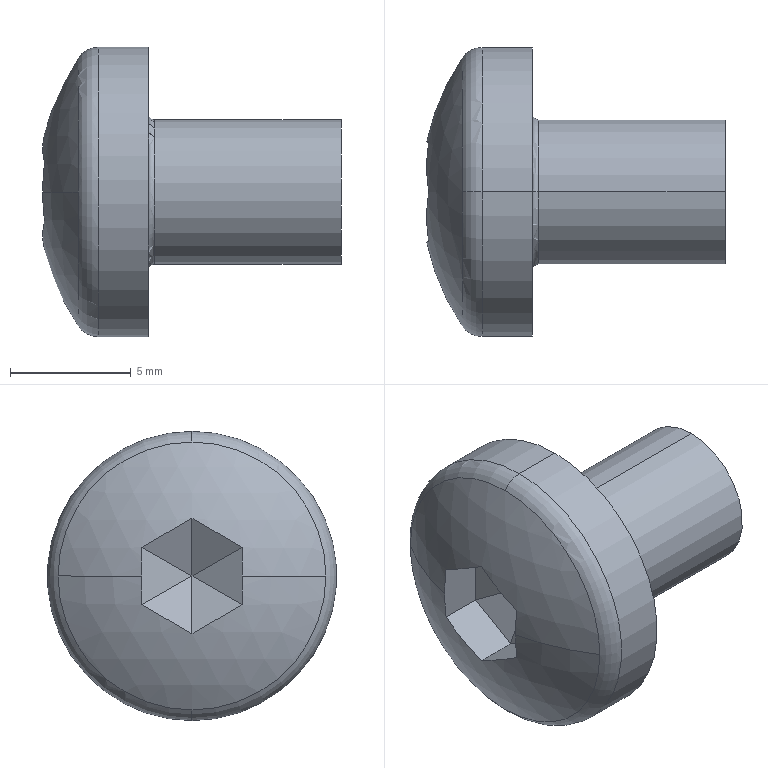Part | SolidWorks | features Cut 2, Fillet 2, RevCut 2, Boss 1, Extrusion 1, LPattern 1 | 1 solid | 24 faces | box 12.382 x 12 x 12 mm | volume 602.281 mm3 | plane 14 | torus 4 | cylinder 4 | sphere 2 | commonest cylinder face diameters 6 x2 12 x2
STEP:
#1=CARTESIAN_POINT('',(1.685,0.,5.556));
#2=VERTEX_POINT('',#1);
#3=CARTESIAN_POINT('',(1.685,5.556,0.));
#4=VERTEX_POINT('',#3);
#5=CARTESIAN_POINT('',(1.685,0.,0.));
#6=DIRECTION('',(-1.,0.,0.));
#7=DIRECTION('',(0.,0.,-1.));
#8=AXIS2_PLACEMENT_3D('',#5,#6,#7);
#9=CIRCLE('',#8,5.556);
#10=EDGE_CURVE('',#2,#4,#9,.T.);
#11=ORIENTED_EDGE('',*,*,#10,.F.);
#12=CARTESIAN_POINT('',(2.517,0.,6.));
#13=VERTEX_POINT('',#12);
#14=CARTESIAN_POINT('',(2.517,0.,5.));
#15=DIRECTION('',(0.,1.,0.));
#16=DIRECTION('',(0.,0.,1.));
#17=AXIS2_PLACEMENT_3D('',#14,#15,#16);
#18=CIRCLE('',#17,1.);
#19=EDGE_CURVE('',#2,#13,#18,.T.);
#20=ORIENTED_EDGE('',*,*,#19,.T.);
#21=CARTESIAN_POINT('',(2.517,0.,-6.));
#22=VERTEX_POINT('',#21);
#23=CARTESIAN_POINT('',(2.517,0.,0.));
#24=DIRECTION('',(1.,0.,0.));
#25=DIRECTION('',(0.,0.,-1.));
#26=AXIS2_PLACEMENT_3D('',#23,#24,#25);
#27=CIRCLE('',#26,6.);
#28=EDGE_CURVE('',#22,#13,#27,.T.);
#29=ORIENTED_EDGE('',*,*,#28,.F.);
#30=CARTESIAN_POINT('',(1.685,0.,-5.556));
#31=VERTEX_POINT('',#30);
#32=CARTESIAN_POINT('',(2.517,0.,-5.));
#33=DIRECTION('',(0.,-1.,0.));
#34=DIRECTION('',(0.,0.,-1.));
#35=AXIS2_PLACEMENT_3D('',#32,#33,#34);
#36=CIRCLE('',#35,1.);
#37=EDGE_CURVE('',#31,#22,#36,.T.);
#38=ORIENTED_EDGE('',*,*,#37,.F.);
#39=CARTESIAN_POINT('',(1.685,0.,0.));
#40=DIRECTION('',(-1.,0.,0.));
#41=DIRECTION('',(0.,0.,-1.));
#42=AXIS2_PLACEMENT_3D('',#39,#40,#41);
#43=CIRCLE('',#42,5.556);
#44=EDGE_CURVE('',#4,#31,#43,.T.);
#45=ORIENTED_EDGE('',*,*,#44,.F.);
#46=EDGE_LOOP('',(#11,#20,#29,#38,#45));
#47=FACE_OUTER_BOUND('',#46,.T.);
#48=CARTESIAN_POINT('',(2.517,0.,0.));
#49=DIRECTION('',(1.,0.,0.));
#50=DIRECTION('',(0.,0.,-1.));
#51=AXIS2_PLACEMENT_3D('',#48,#49,#50);
#52=TOROIDAL_SURFACE('',#51,5.,1.);
#53=ADVANCED_FACE('',(#47),#52,.T.);
#54=CARTESIAN_POINT('',(4.85,0.,3.));
#55=VERTEX_POINT('',#54);
#56=CARTESIAN_POINT('',(4.85,0.,-3.));
#57=VERTEX_POINT('',#56);
#58=CARTESIAN_POINT('',(4.85,0.,0.));
#59=DIRECTION('',(1.,0.,0.));
#60=DIRECTION('',(0.,0.,-1.));
#61=AXIS2_PLACEMENT_3D('',#58,#59,#60);
#62=CIRCLE('',#61,3.);
#63=EDGE_CURVE('',#55,#57,#62,.T.);
#64=ORIENTED_EDGE('',*,*,#63,.F.);
#65=CARTESIAN_POINT('',(4.6,0.,3.25));
#66=VERTEX_POINT('',#65);
#67=CARTESIAN_POINT('',(4.85,0.,3.25));
#68=DIRECTION('',(0.,1.,0.));
#69=DIRECTION('',(0.,0.,1.));
#70=AXIS2_PLACEMENT_3D('',#67,#68,#69);
#71=CIRCLE('',#70,0.25);
#72=EDGE_CURVE('',#55,#66,#71,.T.);
#73=ORIENTED_EDGE('',*,*,#72,.T.);
#74=CARTESIAN_POINT('',(4.6,0.,-3.25));
#75=VERTEX_POINT('',#74);
#76=CARTESIAN_POINT('',(4.6,0.,0.));
#77=DIRECTION('',(-1.,0.,0.));
#78=DIRECTION('',(0.,0.,-1.));
#79=AXIS2_PLACEMENT_3D('',#76,#77,#78);
#80=CIRCLE('',#79,3.25);
#81=EDGE_CURVE('',#75,#66,#80,.T.);
#82=ORIENTED_EDGE('',*,*,#81,.F.);
#83=CARTESIAN_POINT('',(4.85,0.,-3.25));
#84=DIRECTION('',(0.,-1.,0.));
#85=DIRECTION('',(0.,0.,-1.));
#86=AXIS2_PLACEMENT_3D('',#83,#84,#85);
#87=CIRCLE('',#86,0.25);
#88=EDGE_CURVE('',#57,#75,#87,.T.);
#89=ORIENTED_EDGE('',*,*,#88,.F.);
#90=EDGE_LOOP('',(#64,#73,#82,#89));
#91=FACE_OUTER_BOUND('',#90,.T.);
#92=CARTESIAN_POINT('',(4.85,0.,0.));
#93=DIRECTION('',(1.,0.,0.));
#94=DIRECTION('',(0.,0.,-1.));
#95=AXIS2_PLACEMENT_3D('',#92,#93,#94);
#96=TOROIDAL_SURFACE('',#95,3.25,0.25);
#97=ADVANCED_FACE('',(#91),#96,.F.);
#98=CARTESIAN_POINT('',(12.6,0.,-3.));
#99=VERTEX_POINT('',#98);
#100=CARTESIAN_POINT('',(12.6,0.,3.));
#101=VERTEX_POINT('',#100);
#102=CARTESIAN_POINT('',(12.6,0.,0.));
#103=DIRECTION('',(1.,0.,0.));
#104=DIRECTION('',(0.,0.,-1.));
#105=AXIS2_PLACEMENT_3D('',#102,#103,#104);
#106=CIRCLE('',#105,3.);
#107=EDGE_CURVE('',#99,#101,#106,.T.);
#108=ORIENTED_EDGE('',*,*,#107,.F.);
#109=CARTESIAN_POINT('',(12.6,0.,-3.));
#110=DIRECTION('',(-1.,0.,0.));
#111=VECTOR('',#110,1000.);
#112=LINE('',#109,#111);
#113=EDGE_CURVE('',#99,#57,#112,.T.);
#114=ORIENTED_EDGE('',*,*,#113,.T.);
#115=CARTESIAN_POINT('',(4.85,0.,0.));
#116=DIRECTION('',(1.,0.,0.));
#117=DIRECTION('',(0.,0.,-1.));
#118=AXIS2_PLACEMENT_3D('',#115,#116,#117);
#119=CIRCLE('',#118,3.);
#120=EDGE_CURVE('',#57,#55,#119,.T.);
#121=ORIENTED_EDGE('',*,*,#120,.T.);
#122=CARTESIAN_POINT('',(12.6,0.,3.));
#123=DIRECTION('',(-1.,0.,0.));
#124=VECTOR('',#123,1000.);
#125=LINE('',#122,#124);
#126=EDGE_CURVE('',#101,#55,#125,.T.);
#127=ORIENTED_EDGE('',*,*,#126,.F.);
#128=EDGE_LOOP('',(#108,#114,#121,#127));
#129=FACE_OUTER_BOUND('',#128,.T.);
#130=CARTESIAN_POINT('',(12.6,0.,0.));
#131=DIRECTION('',(-1.,0.,0.));
#132=DIRECTION('',(0.,0.,1.));
#133=AXIS2_PLACEMENT_3D('',#130,#131,#132);
#134=CYLINDRICAL_SURFACE('',#133,3.);
#135=ADVANCED_FACE('',(#129),#134,.T.);
#136=CARTESIAN_POINT('',(4.6,0.,-6.));
#137=VERTEX_POINT('',#136);
#138=CARTESIAN_POINT('',(4.6,0.,6.));
#139=VERTEX_POINT('',#138);
#140=CARTESIAN_POINT('',(4.6,0.,0.));
#141=DIRECTION('',(1.,0.,0.));
#142=DIRECTION('',(0.,0.,-1.));
#143=AXIS2_PLACEMENT_3D('',#140,#141,#142);
#144=CIRCLE('',#143,6.);
#145=EDGE_CURVE('',#137,#139,#144,.T.);
#146=ORIENTED_EDGE('',*,*,#145,.F.);
#147=CARTESIAN_POINT('',(4.6,0.,-6.));
#148=DIRECTION('',(-1.,0.,0.));
#149=VECTOR('',#148,1000.);
#150=LINE('',#147,#149);
#151=EDGE_CURVE('',#137,#22,#150,.T.);
#152=ORIENTED_EDGE('',*,*,#151,.T.);
#153=ORIENTED_EDGE('',*,*,#28,.T.);
#154=CARTESIAN_POINT('',(4.6,0.,6.));
#155=DIRECTION('',(-1.,0.,0.));
#156=VECTOR('',#155,1000.);
#157=LINE('',#154,#156);
#158=EDGE_CURVE('',#139,#13,#157,.T.);
#159=ORIENTED_EDGE('',*,*,#158,.F.);
#160=EDGE_LOOP('',(#146,#152,#153,#159));
#161=FACE_OUTER_BOUND('',#160,.T.);
#162=CARTESIAN_POINT('',(4.6,0.,0.));
#163=DIRECTION('',(-1.,0.,0.));
#164=DIRECTION('',(0.,0.,1.));
#165=AXIS2_PLACEMENT_3D('',#162,#163,#164);
#166=CYLINDRICAL_SURFACE('',#165,6.);
#167=ADVANCED_FACE('',(#161),#166,.T.);
#168=CARTESIAN_POINT('',(1.685,-5.556,0.));
#169=VERTEX_POINT('',#168);
#170=CARTESIAN_POINT('',(1.685,0.,0.));
#171=DIRECTION('',(-1.,0.,0.));
#172=DIRECTION('',(0.,0.,-1.));
#173=AXIS2_PLACEMENT_3D('',#170,#171,#172);
#174=CIRCLE('',#173,5.556);
#175=EDGE_CURVE('',#169,#2,#174,.T.);
#176=ORIENTED_EDGE('',*,*,#175,.T.);
#177=ORIENTED_EDGE('',*,*,#10,.T.);
#178=CARTESIAN_POINT('',(0.2176,2.075,0.));
#179=VERTEX_POINT('',#178);
#180=CARTESIAN_POINT('',(10.,0.,0.));
#181=DIRECTION('',(0.,0.,1.));
#182=DIRECTION('',(0.,-1.,0.));
#183=AXIS2_PLACEMENT_3D('',#180,#181,#182);
#184=CIRCLE('',#183,10.);
#185=EDGE_CURVE('',#4,#179,#184,.T.);
#186=ORIENTED_EDGE('',*,*,#185,.T.);
#187=CARTESIAN_POINT('',(0.2913,2.075,1.198));
#188=VERTEX_POINT('',#187);
#189=CARTESIAN_POINT('',(10.,2.075,0.));
#190=DIRECTION('',(0.,1.,0.));
#191=DIRECTION('',(0.,0.,-1.));
#192=AXIS2_PLACEMENT_3D('',#189,#190,#191);
#193=CIRCLE('',#192,9.782);
#194=EDGE_CURVE('',#179,#188,#193,.T.);
#195=ORIENTED_EDGE('',*,*,#194,.T.);
#196=CARTESIAN_POINT('',(0.2913,0.,2.396));
#197=VERTEX_POINT('',#196);
#198=CARTESIAN_POINT('',(10.,1.038,1.797));
#199=DIRECTION('',(0.,0.5,0.866));
#200=DIRECTION('',(0.,0.866,-0.5));
#201=AXIS2_PLACEMENT_3D('',#198,#199,#200);
#202=CIRCLE('',#201,9.782);
#203=EDGE_CURVE('',#188,#197,#202,.T.);
#204=ORIENTED_EDGE('',*,*,#203,.T.);
#205=CARTESIAN_POINT('',(0.2913,-2.075,1.198));
#206=VERTEX_POINT('',#205);
#207=CARTESIAN_POINT('',(10.,-1.037,1.797));
#208=DIRECTION('',(0.,-0.5,0.866));
#209=DIRECTION('',(0.,0.866,0.5));
#210=AXIS2_PLACEMENT_3D('',#207,#208,#209);
#211=CIRCLE('',#210,9.782);
#212=EDGE_CURVE('',#197,#206,#211,.T.);
#213=ORIENTED_EDGE('',*,*,#212,.T.);
#214=CARTESIAN_POINT('',(0.2176,-2.075,0.));
#215=VERTEX_POINT('',#214);
#216=CARTESIAN_POINT('',(10.,-2.075,0.));
#217=DIRECTION('',(0.,-1.,0.));
#218=DIRECTION('',(0.,0.,1.));
#219=AXIS2_PLACEMENT_3D('',#216,#217,#218);
#220=CIRCLE('',#219,9.782);
#221=EDGE_CURVE('',#206,#215,#220,.T.);
#222=ORIENTED_EDGE('',*,*,#221,.T.);
#223=CARTESIAN_POINT('',(10.,0.,0.));
#224=DIRECTION('',(0.,0.,-1.));
#225=DIRECTION('',(-1.,0.,0.));
#226=AXIS2_PLACEMENT_3D('',#223,#224,#225);
#227=CIRCLE('',#226,10.);
#228=EDGE_CURVE('',#169,#215,#227,.T.);
#229=ORIENTED_EDGE('',*,*,#228,.F.);
#230=EDGE_LOOP('',(#176,#177,#186,#195,#204,#213,#222,#229));
#231=FACE_OUTER_BOUND('',#230,.T.);
#232=CARTESIAN_POINT('',(10.,0.,0.));
#233=DIRECTION('',(0.,0.,1.));
#234=DIRECTION('',(0.,-1.,0.));
#235=AXIS2_PLACEMENT_3D('',#232,#233,#234);
#236=SPHERICAL_SURFACE('',#235,10.);
#237=ADVANCED_FACE('',(#231),#236,.T.);
#238=ORIENTED_EDGE('',*,*,#185,.F.);
#239=ORIENTED_EDGE('',*,*,#44,.T.);
#240=CARTESIAN_POINT('',(1.685,0.,0.));
#241=DIRECTION('',(-1.,0.,0.));
#242=DIRECTION('',(0.,0.,-1.));
#243=AXIS2_PLACEMENT_3D('',#240,#241,#242);
#244=CIRCLE('',#243,5.556);
#245=EDGE_CURVE('',#31,#169,#244,.T.);
#246=ORIENTED_EDGE('',*,*,#245,.T.);
#247=ORIENTED_EDGE('',*,*,#228,.T.);
#248=CARTESIAN_POINT('',(0.2913,-2.075,-1.198));
#249=VERTEX_POINT('',#248);
#250=CARTESIAN_POINT('',(10.,-2.075,0.));
#251=DIRECTION('',(0.,-1.,0.));
#252=DIRECTION('',(0.,0.,1.));
#253=AXIS2_PLACEMENT_3D('',#250,#251,#252);
#254=CIRCLE('',#253,9.782);
#255=EDGE_CURVE('',#215,#249,#254,.T.);
#256=ORIENTED_EDGE('',*,*,#255,.T.);
#257=CARTESIAN_POINT('',(0.2913,0.,-2.396));
#258=VERTEX_POINT('',#257);
#259=CARTESIAN_POINT('',(10.,-1.038,-1.797));
#260=DIRECTION('',(0.,-0.5,-0.866));
#261=DIRECTION('',(0.,-0.866,0.5));
#262=AXIS2_PLACEMENT_3D('',#259,#260,#261);
#263=CIRCLE('',#262,9.782);
#264=EDGE_CURVE('',#249,#258,#263,.T.);
#265=ORIENTED_EDGE('',*,*,#264,.T.);
#266=CARTESIAN_POINT('',(0.2913,2.075,-1.198));
#267=VERTEX_POINT('',#266);
#268=CARTESIAN_POINT('',(10.,1.037,-1.797));
#269=DIRECTION('',(0.,0.5,-0.866));
#270=DIRECTION('',(0.,-0.866,-0.5));
#271=AXIS2_PLACEMENT_3D('',#268,#269,#270);
#272=CIRCLE('',#271,9.782);
#273=EDGE_CURVE('',#258,#267,#272,.T.);
#274=ORIENTED_EDGE('',*,*,#273,.T.);
#275=CARTESIAN_POINT('',(10.,2.075,0.));
#276=DIRECTION('',(0.,1.,0.));
#277=DIRECTION('',(0.,0.,-1.));
#278=AXIS2_PLACEMENT_3D('',#275,#276,#277);
#279=CIRCLE('',#278,9.782);
#280=EDGE_CURVE('',#267,#179,#279,.T.);
#281=ORIENTED_EDGE('',*,*,#280,.T.);
#282=EDGE_LOOP('',(#238,#239,#246,#247,#256,#265,#274,#281));
#283=FACE_OUTER_BOUND('',#282,.T.);
#284=CARTESIAN_POINT('',(10.,0.,0.));
#285=DIRECTION('',(0.,0.,1.));
#286=DIRECTION('',(0.,-1.,0.));
#287=AXIS2_PLACEMENT_3D('',#284,#285,#286);
#288=SPHERICAL_SURFACE('',#287,10.);
#289=ADVANCED_FACE('',(#283),#288,.T.);
#290=ORIENTED_EDGE('',*,*,#151,.F.);
#291=CARTESIAN_POINT('',(4.6,0.,0.));
#292=DIRECTION('',(1.,0.,0.));
#293=DIRECTION('',(0.,0.,-1.));
#294=AXIS2_PLACEMENT_3D('',#291,#292,#293);
#295=CIRCLE('',#294,6.);
#296=EDGE_CURVE('',#139,#137,#295,.T.);
#297=ORIENTED_EDGE('',*,*,#296,.F.);
#298=ORIENTED_EDGE('',*,*,#158,.T.);
#299=CARTESIAN_POINT('',(2.517,0.,0.));
#300=DIRECTION('',(1.,0.,0.));
#301=DIRECTION('',(0.,0.,-1.));
#302=AXIS2_PLACEMENT_3D('',#299,#300,#301);
#303=CIRCLE('',#302,6.);
#304=EDGE_CURVE('',#13,#22,#303,.T.);
#305=ORIENTED_EDGE('',*,*,#304,.T.);
#306=EDGE_LOOP('',(#290,#297,#298,#305));
#307=FACE_OUTER_BOUND('',#306,.T.);
#308=CARTESIAN_POINT('',(4.6,0.,0.));
#309=DIRECTION('',(-1.,0.,0.));
#310=DIRECTION('',(0.,0.,1.));
#311=AXIS2_PLACEMENT_3D('',#308,#309,#310);
#312=CYLINDRICAL_SURFACE('',#311,6.);
#313=ADVANCED_FACE('',(#307),#312,.T.);
#314=ORIENTED_EDGE('',*,*,#81,.T.);
#315=CARTESIAN_POINT('',(4.6,0.,0.));
#316=DIRECTION('',(-1.,0.,0.));
#317=DIRECTION('',(0.,0.,-1.));
#318=AXIS2_PLACEMENT_3D('',#315,#316,#317);
#319=CIRCLE('',#318,3.25);
#320=EDGE_CURVE('',#66,#75,#319,.T.);
#321=ORIENTED_EDGE('',*,*,#320,.T.);
#322=EDGE_LOOP('',(#314,#321));
#323=FACE_BOUND('',#322,.T.);
#324=ORIENTED_EDGE('',*,*,#296,.T.);
#325=ORIENTED_EDGE('',*,*,#145,.T.);
#326=EDGE_LOOP('',(#324,#325));
#327=FACE_OUTER_BOUND('',#326,.T.);
#328=CARTESIAN_POINT('',(4.6,0.,0.));
#329=DIRECTION('',(1.,0.,0.));
#330=DIRECTION('',(0.,0.,-1.));
#331=AXIS2_PLACEMENT_3D('',#328,#329,#330);
#332=PLANE('',#331);
#333=ADVANCED_FACE('',(#323,#327),#332,.T.);
#334=ORIENTED_EDGE('',*,*,#113,.F.);
#335=CARTESIAN_POINT('',(12.6,0.,0.));
#336=DIRECTION('',(1.,0.,0.));
#337=DIRECTION('',(0.,0.,-1.));
#338=AXIS2_PLACEMENT_3D('',#335,#336,#337);
#339=CIRCLE('',#338,3.);
#340=EDGE_CURVE('',#101,#99,#339,.T.);
#341=ORIENTED_EDGE('',*,*,#340,.F.);
#342=ORIENTED_EDGE('',*,*,#126,.T.);
#343=ORIENTED_EDGE('',*,*,#63,.T.);
#344=EDGE_LOOP('',(#334,#341,#342,#343));
#345=FACE_OUTER_BOUND('',#344,.T.);
#346=CARTESIAN_POINT('',(12.6,0.,0.));
#347=DIRECTION('',(-1.,0.,0.));
#348=DIRECTION('',(0.,0.,1.));
#349=AXIS2_PLACEMENT_3D('',#346,#347,#348);
#350=CYLINDRICAL_SURFACE('',#349,3.);
#351=ADVANCED_FACE('',(#345),#350,.T.);
#352=ORIENTED_EDGE('',*,*,#340,.T.);
#353=ORIENTED_EDGE('',*,*,#107,.T.);
#354=EDGE_LOOP('',(#352,#353));
#355=FACE_OUTER_BOUND('',#354,.T.);
#356=CARTESIAN_POINT('',(12.6,0.,0.));
#357=DIRECTION('',(1.,0.,0.));
#358=DIRECTION('',(0.,0.,-1.));
#359=AXIS2_PLACEMENT_3D('',#356,#357,#358);
#360=PLANE('',#359);
#361=ADVANCED_FACE('',(#355),#360,.T.);
#362=ORIENTED_EDGE('',*,*,#72,.F.);
#363=ORIENTED_EDGE('',*,*,#120,.F.);
#364=ORIENTED_EDGE('',*,*,#88,.T.);
#365=ORIENTED_EDGE('',*,*,#320,.F.);
#366=EDGE_LOOP('',(#362,#363,#364,#365));
#367=FACE_OUTER_BOUND('',#366,.T.);
#368=CARTESIAN_POINT('',(4.85,0.,0.));
#369=DIRECTION('',(1.,0.,0.));
#370=DIRECTION('',(0.,0.,-1.));
#371=AXIS2_PLACEMENT_3D('',#368,#369,#370);
#372=TOROIDAL_SURFACE('',#371,3.25,0.25);
#373=ADVANCED_FACE('',(#367),#372,.F.);
#374=CARTESIAN_POINT('',(2.,-2.075,-1.198));
#375=VERTEX_POINT('',#374);
#376=CARTESIAN_POINT('',(2.,-2.075,-1.198));
#377=DIRECTION('',(-1.,0.,0.));
#378=VECTOR('',#377,1000.);
#379=LINE('',#376,#378);
#380=EDGE_CURVE('',#375,#249,#379,.T.);
#381=ORIENTED_EDGE('',*,*,#380,.F.);
#382=CARTESIAN_POINT('',(2.,0.,-2.396));
#383=VERTEX_POINT('',#382);
#384=CARTESIAN_POINT('',(2.,-2.075,-1.198));
#385=DIRECTION('',(0.,0.866,-0.5));
#386=VECTOR('',#385,1000.);
#387=LINE('',#384,#386);
#388=EDGE_CURVE('',#375,#383,#387,.T.);
#389=ORIENTED_EDGE('',*,*,#388,.T.);
#390=CARTESIAN_POINT('',(2.,0.,-2.396));
#391=DIRECTION('',(-1.,0.,0.));
#392=VECTOR('',#391,1000.);
#393=LINE('',#390,#392);
#394=EDGE_CURVE('',#383,#258,#393,.T.);
#395=ORIENTED_EDGE('',*,*,#394,.T.);
#396=ORIENTED_EDGE('',*,*,#264,.F.);
#397=EDGE_LOOP('',(#381,#389,#395,#396));
#398=FACE_OUTER_BOUND('',#397,.T.);
#399=CARTESIAN_POINT('',(2.,-2.075,-1.198));
#400=DIRECTION('',(0.,0.5,0.866));
#401=DIRECTION('',(0.,-0.866,0.5));
#402=AXIS2_PLACEMENT_3D('',#399,#400,#401);
#403=PLANE('',#402);
#404=ADVANCED_FACE('',(#398),#403,.T.);
#405=ORIENTED_EDGE('',*,*,#394,.F.);
#406=CARTESIAN_POINT('',(2.,2.075,-1.198));
#407=VERTEX_POINT('',#406);
#408=CARTESIAN_POINT('',(2.,0.,-2.396));
#409=DIRECTION('',(0.,0.866,0.5));
#410=VECTOR('',#409,1000.);
#411=LINE('',#408,#410);
#412=EDGE_CURVE('',#383,#407,#411,.T.);
#413=ORIENTED_EDGE('',*,*,#412,.T.);
#414=CARTESIAN_POINT('',(2.,2.075,-1.198));
#415=DIRECTION('',(-1.,0.,0.));
#416=VECTOR('',#415,1000.);
#417=LINE('',#414,#416);
#418=EDGE_CURVE('',#407,#267,#417,.T.);
#419=ORIENTED_EDGE('',*,*,#418,.T.);
#420=ORIENTED_EDGE('',*,*,#273,.F.);
#421=EDGE_LOOP('',(#405,#413,#419,#420));
#422=FACE_OUTER_BOUND('',#421,.T.);
#423=CARTESIAN_POINT('',(2.,0.,-2.396));
#424=DIRECTION('',(0.,-0.5,0.866));
#425=DIRECTION('',(0.,-0.866,-0.5));
#426=AXIS2_PLACEMENT_3D('',#423,#424,#425);
#427=PLANE('',#426);
#428=ADVANCED_FACE('',(#422),#427,.T.);
#429=ORIENTED_EDGE('',*,*,#418,.F.);
#430=CARTESIAN_POINT('',(2.,2.075,1.198));
#431=VERTEX_POINT('',#430);
#432=CARTESIAN_POINT('',(2.,2.075,-1.198));
#433=DIRECTION('',(0.,0.,1.));
#434=VECTOR('',#433,1000.);
#435=LINE('',#432,#434);
#436=EDGE_CURVE('',#407,#431,#435,.T.);
#437=ORIENTED_EDGE('',*,*,#436,.T.);
#438=CARTESIAN_POINT('',(2.,2.075,1.198));
#439=DIRECTION('',(-1.,0.,0.));
#440=VECTOR('',#439,1000.);
#441=LINE('',#438,#440);
#442=EDGE_CURVE('',#431,#188,#441,.T.);
#443=ORIENTED_EDGE('',*,*,#442,.T.);
#444=ORIENTED_EDGE('',*,*,#194,.F.);
#445=ORIENTED_EDGE('',*,*,#280,.F.);
#446=EDGE_LOOP('',(#429,#437,#443,#444,#445));
#447=FACE_OUTER_BOUND('',#446,.T.);
#448=CARTESIAN_POINT('',(2.,2.075,-1.198));
#449=DIRECTION('',(0.,-1.,0.));
#450=DIRECTION('',(0.,0.,-1.));
#451=AXIS2_PLACEMENT_3D('',#448,#449,#450);
#452=PLANE('',#451);
#453=ADVANCED_FACE('',(#447),#452,.T.);
#454=ORIENTED_EDGE('',*,*,#442,.F.);
#455=CARTESIAN_POINT('',(2.,0.,2.396));
#456=VERTEX_POINT('',#455);
#457=CARTESIAN_POINT('',(2.,2.075,1.198));
#458=DIRECTION('',(0.,-0.866,0.5));
#459=VECTOR('',#458,1000.);
#460=LINE('',#457,#459);
#461=EDGE_CURVE('',#431,#456,#460,.T.);
#462=ORIENTED_EDGE('',*,*,#461,.T.);
#463=CARTESIAN_POINT('',(2.,0.,2.396));
#464=DIRECTION('',(-1.,0.,0.));
#465=VECTOR('',#464,1000.);
#466=LINE('',#463,#465);
#467=EDGE_CURVE('',#456,#197,#466,.T.);
#468=ORIENTED_EDGE('',*,*,#467,.T.);
#469=ORIENTED_EDGE('',*,*,#203,.F.);
#470=EDGE_LOOP('',(#454,#462,#468,#469));
#471=FACE_OUTER_BOUND('',#470,.T.);
#472=CARTESIAN_POINT('',(2.,2.075,1.198));
#473=DIRECTION('',(0.,-0.5,-0.866));
#474=DIRECTION('',(0.,0.866,-0.5));
#475=AXIS2_PLACEMENT_3D('',#472,#473,#474);
#476=PLANE('',#475);
#477=ADVANCED_FACE('',(#471),#476,.T.);
#478=ORIENTED_EDGE('',*,*,#467,.F.);
#479=CARTESIAN_POINT('',(2.,-2.075,1.198));
#480=VERTEX_POINT('',#479);
#481=CARTESIAN_POINT('',(2.,0.,2.396));
#482=DIRECTION('',(0.,-0.866,-0.5));
#483=VECTOR('',#482,1000.);
#484=LINE('',#481,#483);
#485=EDGE_CURVE('',#456,#480,#484,.T.);
#486=ORIENTED_EDGE('',*,*,#485,.T.);
#487=CARTESIAN_POINT('',(2.,-2.075,1.198));
#488=DIRECTION('',(-1.,0.,0.));
#489=VECTOR('',#488,1000.);
#490=LINE('',#487,#489);
#491=EDGE_CURVE('',#480,#206,#490,.T.);
#492=ORIENTED_EDGE('',*,*,#491,.T.);
#493=ORIENTED_EDGE('',*,*,#212,.F.);
#494=EDGE_LOOP('',(#478,#486,#492,#493));
#495=FACE_OUTER_BOUND('',#494,.T.);
#496=CARTESIAN_POINT('',(2.,0.,2.396));
#497=DIRECTION('',(0.,0.5,-0.866));
#498=DIRECTION('',(0.,0.866,0.5));
#499=AXIS2_PLACEMENT_3D('',#496,#497,#498);
#500=PLANE('',#499);
#501=ADVANCED_FACE('',(#495),#500,.T.);
#502=ORIENTED_EDGE('',*,*,#491,.F.);
#503=CARTESIAN_POINT('',(2.,-2.075,1.198));
#504=DIRECTION('',(0.,0.,-1.));
#505=VECTOR('',#504,1000.);
#506=LINE('',#503,#505);
#507=EDGE_CURVE('',#480,#375,#506,.T.);
#508=ORIENTED_EDGE('',*,*,#507,.T.);
#509=ORIENTED_EDGE('',*,*,#380,.T.);
#510=ORIENTED_EDGE('',*,*,#255,.F.);
#511=ORIENTED_EDGE('',*,*,#221,.F.);
#512=EDGE_LOOP('',(#502,#508,#509,#510,#511));
#513=FACE_OUTER_BOUND('',#512,.T.);
#514=CARTESIAN_POINT('',(2.,-2.075,1.198));
#515=DIRECTION('',(0.,1.,0.));
#516=DIRECTION('',(0.,0.,1.));
#517=AXIS2_PLACEMENT_3D('',#514,#515,#516);
#518=PLANE('',#517);
#519=ADVANCED_FACE('',(#513),#518,.T.);
#520=ORIENTED_EDGE('',*,*,#461,.F.);
#521=CARTESIAN_POINT('',(3.198,0.,0.));
#522=VERTEX_POINT('',#521);
#523=CARTESIAN_POINT('',(2.,2.075,1.198));
#524=DIRECTION('',(-0.4472,0.7746,0.4472));
#525=VECTOR('',#524,1000.);
#526=LINE('',#523,#525);
#527=EDGE_CURVE('',#522,#431,#526,.T.);
#528=ORIENTED_EDGE('',*,*,#527,.F.);
#529=CARTESIAN_POINT('',(2.,0.,2.396));
#530=DIRECTION('',(-0.4472,0.,0.8944));
#531=VECTOR('',#530,1000.);
#532=LINE('',#529,#531);
#533=EDGE_CURVE('',#522,#456,#532,.T.);
#534=ORIENTED_EDGE('',*,*,#533,.T.);
#535=EDGE_LOOP('',(#520,#528,#534));
#536=FACE_OUTER_BOUND('',#535,.T.);
#537=CARTESIAN_POINT('',(2.,2.075,1.198));
#538=DIRECTION('',(0.866,0.25,0.433));
#539=DIRECTION('',(0.4472,0.,-0.8944));
#540=AXIS2_PLACEMENT_3D('',#537,#538,#539);
#541=PLANE('',#540);
#542=ADVANCED_FACE('',(#536),#541,.F.);
#543=ORIENTED_EDGE('',*,*,#485,.F.);
#544=ORIENTED_EDGE('',*,*,#533,.F.);
#545=CARTESIAN_POINT('',(2.,-2.075,1.198));
#546=DIRECTION('',(-0.4472,-0.7746,0.4472));
#547=VECTOR('',#546,1000.);
#548=LINE('',#545,#547);
#549=EDGE_CURVE('',#522,#480,#548,.T.);
#550=ORIENTED_EDGE('',*,*,#549,.T.);
#551=EDGE_LOOP('',(#543,#544,#550));
#552=FACE_OUTER_BOUND('',#551,.T.);
#553=CARTESIAN_POINT('',(2.,0.,2.396));
#554=DIRECTION('',(0.866,-0.25,0.433));
#555=DIRECTION('',(0.4472,0.,-0.8944));
#556=AXIS2_PLACEMENT_3D('',#553,#554,#555);
#557=PLANE('',#556);
#558=ADVANCED_FACE('',(#552),#557,.F.);
#559=ORIENTED_EDGE('',*,*,#507,.F.);
#560=ORIENTED_EDGE('',*,*,#549,.F.);
#561=CARTESIAN_POINT('',(2.,-2.075,-1.198));
#562=DIRECTION('',(-0.4472,-0.7746,-0.4472));
#563=VECTOR('',#562,1000.);
#564=LINE('',#561,#563);
#565=EDGE_CURVE('',#522,#375,#564,.T.);
#566=ORIENTED_EDGE('',*,*,#565,.T.);
#567=EDGE_LOOP('',(#559,#560,#566));
#568=FACE_OUTER_BOUND('',#567,.T.);
#569=CARTESIAN_POINT('',(2.,-2.075,1.198));
#570=DIRECTION('',(0.866,-0.5,0.));
#571=DIRECTION('',(0.5,0.866,0.));
#572=AXIS2_PLACEMENT_3D('',#569,#570,#571);
#573=PLANE('',#572);
#574=ADVANCED_FACE('',(#568),#573,.F.);
#575=ORIENTED_EDGE('',*,*,#388,.F.);
#576=ORIENTED_EDGE('',*,*,#565,.F.);
#577=CARTESIAN_POINT('',(2.,0.,-2.396));
#578=DIRECTION('',(-0.4472,0.,-0.8944));
#579=VECTOR('',#578,1000.);
#580=LINE('',#577,#579);
#581=EDGE_CURVE('',#522,#383,#580,.T.);
#582=ORIENTED_EDGE('',*,*,#581,.T.);
#583=EDGE_LOOP('',(#575,#576,#582));
#584=FACE_OUTER_BOUND('',#583,.T.);
#585=CARTESIAN_POINT('',(2.,-2.075,-1.198));
#586=DIRECTION('',(0.866,-0.25,-0.433));
#587=DIRECTION('',(-0.4472,0.,-0.8944));
#588=AXIS2_PLACEMENT_3D('',#585,#586,#587);
#589=PLANE('',#588);
#590=ADVANCED_FACE('',(#584),#589,.F.);
#591=ORIENTED_EDGE('',*,*,#412,.F.);
#592=ORIENTED_EDGE('',*,*,#581,.F.);
#593=CARTESIAN_POINT('',(2.,2.075,-1.198));
#594=DIRECTION('',(-0.4472,0.7746,-0.4472));
#595=VECTOR('',#594,1000.);
#596=LINE('',#593,#595);
#597=EDGE_CURVE('',#522,#407,#596,.T.);
#598=ORIENTED_EDGE('',*,*,#597,.T.);
#599=EDGE_LOOP('',(#591,#592,#598));
#600=FACE_OUTER_BOUND('',#599,.T.);
#601=CARTESIAN_POINT('',(2.,0.,-2.396));
#602=DIRECTION('',(0.866,0.25,-0.433));
#603=DIRECTION('',(-0.4472,0.,-0.8944));
#604=AXIS2_PLACEMENT_3D('',#601,#602,#603);
#605=PLANE('',#604);
#606=ADVANCED_FACE('',(#600),#605,.F.);
#607=ORIENTED_EDGE('',*,*,#436,.F.);
#608=ORIENTED_EDGE('',*,*,#597,.F.);
#609=ORIENTED_EDGE('',*,*,#527,.T.);
#610=EDGE_LOOP('',(#607,#608,#609));
#611=FACE_OUTER_BOUND('',#610,.T.);
#612=CARTESIAN_POINT('',(2.,2.075,-1.198));
#613=DIRECTION('',(0.866,0.5,0.));
#614=DIRECTION('',(-0.5,0.866,0.));
#615=AXIS2_PLACEMENT_3D('',#612,#613,#614);
#616=PLANE('',#615);
#617=ADVANCED_FACE('',(#611),#616,.F.);
#618=ORIENTED_EDGE('',*,*,#19,.F.);
#619=ORIENTED_EDGE('',*,*,#175,.F.);
#620=ORIENTED_EDGE('',*,*,#245,.F.);
#621=ORIENTED_EDGE('',*,*,#37,.T.);
#622=ORIENTED_EDGE('',*,*,#304,.F.);
#623=EDGE_LOOP('',(#618,#619,#620,#621,#622));
#624=FACE_OUTER_BOUND('',#623,.T.);
#625=CARTESIAN_POINT('',(2.517,0.,0.));
#626=DIRECTION('',(1.,0.,0.));
#627=DIRECTION('',(0.,0.,-1.));
#628=AXIS2_PLACEMENT_3D('',#625,#626,#627);
#629=TOROIDAL_SURFACE('',#628,5.,1.);
#630=ADVANCED_FACE('',(#624),#629,.T.);
#631=CLOSED_SHELL('',(#53,#97,#135,#167,#237,#289,#313,#333,#351,#361,#373,#404,#428,#453,#477,#501,#519,#542,#558,#574,#590,#606,#617,#630));
#632=MANIFOLD_SOLID_BREP('',#631);
#633=CARTESIAN_POINT('',(0.,0.,0.));
#634=DIRECTION('',(0.,0.,1.));
#635=DIRECTION('',(1.,0.,0.));
#636=AXIS2_PLACEMENT_3D('',#633,#634,#635);
#637=(LENGTH_UNIT()NAMED_UNIT(*)SI_UNIT(.MILLI.,.METRE.));
#638=UNCERTAINTY_MEASURE_WITH_UNIT(LENGTH_MEASURE(0.00001),#637,'','');
#639=(NAMED_UNIT(*)PLANE_ANGLE_UNIT()SI_UNIT($,.RADIAN.));
#640=(NAMED_UNIT(*)SI_UNIT($,.STERADIAN.)SOLID_ANGLE_UNIT());
#641=(GEOMETRIC_REPRESENTATION_CONTEXT(3)GLOBAL_UNCERTAINTY_ASSIGNED_CONTEXT((#638))GLOBAL_UNIT_ASSIGNED_CONTEXT((#637,#639,#640))REPRESENTATION_CONTEXT('',''));
#642=ADVANCED_BREP_SHAPE_REPRESENTATION('',(#632,#636),#641);